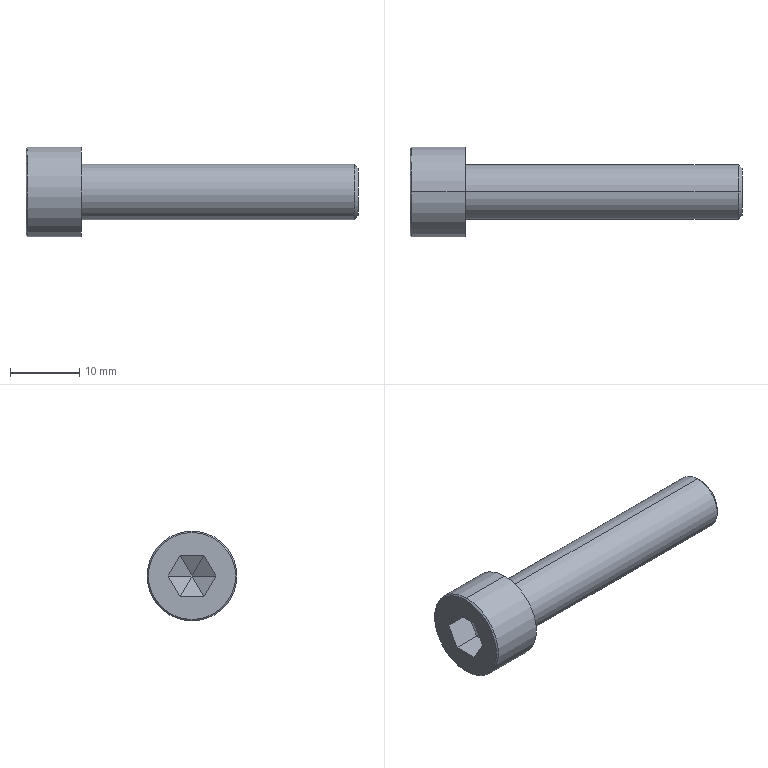Part | NX | features BREP 1 | 1 solid | 23 faces | box 48 x 13 x 13 mm | volume 2924 mm3 | plane 15 | cone 4 | cylinder 4 | commonest cylinder face diameters 8 x2 13 x2
STEP:
#1=CARTESIAN_POINT('',(48.,0.,-3.44));
#2=VERTEX_POINT('',#1);
#3=CARTESIAN_POINT('',(48.,0.,3.44));
#4=VERTEX_POINT('',#3);
#5=CARTESIAN_POINT('',(48.,0.,0.));
#6=DIRECTION('',(1.,0.,0.));
#7=DIRECTION('',(0.,0.,1.));
#8=AXIS2_PLACEMENT_3D('',#5,#6,#7);
#9=CIRCLE('',#8,3.44);
#10=EDGE_CURVE('',#2,#4,#9,.T.);
#11=ORIENTED_EDGE('',*,*,#10,.F.);
#12=CARTESIAN_POINT('',(47.44,0.,-4.));
#13=VERTEX_POINT('',#12);
#14=CARTESIAN_POINT('',(47.44,0.,-4.));
#15=DIRECTION('',(-0.7071,0.,-0.7071));
#16=VECTOR('',#15,1000.);
#17=LINE('',#14,#16);
#18=EDGE_CURVE('',#2,#13,#17,.T.);
#19=ORIENTED_EDGE('',*,*,#18,.T.);
#20=CARTESIAN_POINT('',(47.44,0.,4.));
#21=VERTEX_POINT('',#20);
#22=CARTESIAN_POINT('',(47.44,0.,0.));
#23=DIRECTION('',(-1.,0.,0.));
#24=DIRECTION('',(0.,0.,1.));
#25=AXIS2_PLACEMENT_3D('',#22,#23,#24);
#26=CIRCLE('',#25,4.);
#27=EDGE_CURVE('',#21,#13,#26,.T.);
#28=ORIENTED_EDGE('',*,*,#27,.F.);
#29=CARTESIAN_POINT('',(47.44,0.,4.));
#30=DIRECTION('',(-0.7071,0.,0.7071));
#31=VECTOR('',#30,1000.);
#32=LINE('',#29,#31);
#33=EDGE_CURVE('',#4,#21,#32,.T.);
#34=ORIENTED_EDGE('',*,*,#33,.F.);
#35=EDGE_LOOP('',(#11,#19,#28,#34));
#36=FACE_BOUND('',#35,.T.);
#37=CARTESIAN_POINT('',(47.44,0.,0.));
#38=DIRECTION('',(-1.,0.,0.));
#39=DIRECTION('',(0.,0.,-1.));
#40=AXIS2_PLACEMENT_3D('',#37,#38,#39);
#41=CONICAL_SURFACE('',#40,4.,0.7854);
#42=ADVANCED_FACE('',(#36),#41,.T.);
#43=CARTESIAN_POINT('',(0.,0.,6.3));
#44=VERTEX_POINT('',#43);
#45=CARTESIAN_POINT('',(0.,0.,-6.3));
#46=VERTEX_POINT('',#45);
#47=CARTESIAN_POINT('',(0.,0.,0.));
#48=DIRECTION('',(-1.,0.,0.));
#49=DIRECTION('',(0.,0.,-1.));
#50=AXIS2_PLACEMENT_3D('',#47,#48,#49);
#51=CIRCLE('',#50,6.3);
#52=EDGE_CURVE('',#44,#46,#51,.T.);
#53=ORIENTED_EDGE('',*,*,#52,.F.);
#54=CARTESIAN_POINT('',(0.2,0.,6.5));
#55=VERTEX_POINT('',#54);
#56=CARTESIAN_POINT('',(0.,0.,6.3));
#57=DIRECTION('',(0.7071,0.,0.7071));
#58=VECTOR('',#57,1000.);
#59=LINE('',#56,#58);
#60=EDGE_CURVE('',#55,#44,#59,.F.);
#61=ORIENTED_EDGE('',*,*,#60,.F.);
#62=CARTESIAN_POINT('',(0.2,0.,-6.5));
#63=VERTEX_POINT('',#62);
#64=CARTESIAN_POINT('',(0.2,0.,0.));
#65=DIRECTION('',(1.,0.,0.));
#66=DIRECTION('',(0.,0.,-1.));
#67=AXIS2_PLACEMENT_3D('',#64,#65,#66);
#68=CIRCLE('',#67,6.5);
#69=EDGE_CURVE('',#63,#55,#68,.T.);
#70=ORIENTED_EDGE('',*,*,#69,.F.);
#71=CARTESIAN_POINT('',(0.,0.,-6.3));
#72=DIRECTION('',(0.7071,0.,-0.7071));
#73=VECTOR('',#72,1000.);
#74=LINE('',#71,#73);
#75=EDGE_CURVE('',#63,#46,#74,.F.);
#76=ORIENTED_EDGE('',*,*,#75,.T.);
#77=EDGE_LOOP('',(#53,#61,#70,#76));
#78=FACE_BOUND('',#77,.T.);
#79=CARTESIAN_POINT('',(0.,0.,0.));
#80=DIRECTION('',(1.,0.,0.));
#81=DIRECTION('',(0.,0.,1.));
#82=AXIS2_PLACEMENT_3D('',#79,#80,#81);
#83=CONICAL_SURFACE('',#82,6.3,0.7854);
#84=ADVANCED_FACE('',(#78),#83,.T.);
#85=ORIENTED_EDGE('',*,*,#27,.T.);
#86=CARTESIAN_POINT('',(8.,0.,-4.));
#87=VERTEX_POINT('',#86);
#88=CARTESIAN_POINT('',(0.,0.,-4.));
#89=DIRECTION('',(-1.,0.,0.));
#90=VECTOR('',#89,1000.);
#91=LINE('',#88,#90);
#92=EDGE_CURVE('',#13,#87,#91,.T.);
#93=ORIENTED_EDGE('',*,*,#92,.T.);
#94=CARTESIAN_POINT('',(8.,0.,4.));
#95=VERTEX_POINT('',#94);
#96=CARTESIAN_POINT('',(8.,0.,0.));
#97=DIRECTION('',(-1.,0.,0.));
#98=DIRECTION('',(0.,0.,1.));
#99=AXIS2_PLACEMENT_3D('',#96,#97,#98);
#100=CIRCLE('',#99,4.);
#101=EDGE_CURVE('',#95,#87,#100,.T.);
#102=ORIENTED_EDGE('',*,*,#101,.F.);
#103=CARTESIAN_POINT('',(0.,0.,4.));
#104=DIRECTION('',(-1.,0.,0.));
#105=VECTOR('',#104,1000.);
#106=LINE('',#103,#105);
#107=EDGE_CURVE('',#21,#95,#106,.T.);
#108=ORIENTED_EDGE('',*,*,#107,.F.);
#109=EDGE_LOOP('',(#85,#93,#102,#108));
#110=FACE_BOUND('',#109,.T.);
#111=CARTESIAN_POINT('',(0.,0.,0.));
#112=DIRECTION('',(-1.,0.,0.));
#113=DIRECTION('',(0.,0.,-1.));
#114=AXIS2_PLACEMENT_3D('',#111,#112,#113);
#115=CYLINDRICAL_SURFACE('',#114,4.);
#116=ADVANCED_FACE('',(#110),#115,.T.);
#117=CARTESIAN_POINT('',(8.,0.,6.5));
#118=VERTEX_POINT('',#117);
#119=CARTESIAN_POINT('',(8.,0.,-6.5));
#120=VERTEX_POINT('',#119);
#121=CARTESIAN_POINT('',(8.,0.,0.));
#122=DIRECTION('',(-1.,0.,0.));
#123=DIRECTION('',(0.,0.,1.));
#124=AXIS2_PLACEMENT_3D('',#121,#122,#123);
#125=CIRCLE('',#124,6.5);
#126=EDGE_CURVE('',#118,#120,#125,.T.);
#127=ORIENTED_EDGE('',*,*,#126,.T.);
#128=CARTESIAN_POINT('',(0.,0.,-6.5));
#129=DIRECTION('',(-1.,0.,0.));
#130=VECTOR('',#129,1000.);
#131=LINE('',#128,#130);
#132=EDGE_CURVE('',#120,#63,#131,.T.);
#133=ORIENTED_EDGE('',*,*,#132,.T.);
#134=ORIENTED_EDGE('',*,*,#69,.T.);
#135=CARTESIAN_POINT('',(0.,0.,6.5));
#136=DIRECTION('',(-1.,0.,0.));
#137=VECTOR('',#136,1000.);
#138=LINE('',#135,#137);
#139=EDGE_CURVE('',#118,#55,#138,.T.);
#140=ORIENTED_EDGE('',*,*,#139,.F.);
#141=EDGE_LOOP('',(#127,#133,#134,#140));
#142=FACE_BOUND('',#141,.T.);
#143=CARTESIAN_POINT('',(0.,0.,0.));
#144=DIRECTION('',(-1.,0.,0.));
#145=DIRECTION('',(0.,0.,-1.));
#146=AXIS2_PLACEMENT_3D('',#143,#144,#145);
#147=CYLINDRICAL_SURFACE('',#146,6.5);
#148=ADVANCED_FACE('',(#142),#147,.T.);
#149=CARTESIAN_POINT('',(0.,0.,0.));
#150=DIRECTION('',(-1.,0.,0.));
#151=DIRECTION('',(0.,0.,-1.));
#152=AXIS2_PLACEMENT_3D('',#149,#150,#151);
#153=CIRCLE('',#152,6.3);
#154=EDGE_CURVE('',#46,#44,#153,.T.);
#155=ORIENTED_EDGE('',*,*,#154,.T.);
#156=ORIENTED_EDGE('',*,*,#52,.T.);
#157=EDGE_LOOP('',(#155,#156));
#158=FACE_BOUND('',#157,.T.);
#159=CARTESIAN_POINT('',(0.,1.732,-3.));
#160=VERTEX_POINT('',#159);
#161=CARTESIAN_POINT('',(0.,3.464,0.));
#162=VERTEX_POINT('',#161);
#163=CARTESIAN_POINT('',(0.,1.732,-3.));
#164=DIRECTION('',(0.,0.5,0.866));
#165=VECTOR('',#164,1000.);
#166=LINE('',#163,#165);
#167=EDGE_CURVE('',#160,#162,#166,.T.);
#168=ORIENTED_EDGE('',*,*,#167,.T.);
#169=CARTESIAN_POINT('',(0.,1.732,3.));
#170=VERTEX_POINT('',#169);
#171=CARTESIAN_POINT('',(0.,3.464,0.));
#172=DIRECTION('',(0.,-0.5,0.866));
#173=VECTOR('',#172,1000.);
#174=LINE('',#171,#173);
#175=EDGE_CURVE('',#162,#170,#174,.T.);
#176=ORIENTED_EDGE('',*,*,#175,.T.);
#177=CARTESIAN_POINT('',(0.,-1.732,3.));
#178=VERTEX_POINT('',#177);
#179=CARTESIAN_POINT('',(0.,1.732,3.));
#180=DIRECTION('',(0.,-1.,0.));
#181=VECTOR('',#180,1000.);
#182=LINE('',#179,#181);
#183=EDGE_CURVE('',#170,#178,#182,.T.);
#184=ORIENTED_EDGE('',*,*,#183,.T.);
#185=CARTESIAN_POINT('',(0.,-3.464,0.));
#186=VERTEX_POINT('',#185);
#187=CARTESIAN_POINT('',(0.,-1.732,3.));
#188=DIRECTION('',(0.,-0.5,-0.866));
#189=VECTOR('',#188,1000.);
#190=LINE('',#187,#189);
#191=EDGE_CURVE('',#178,#186,#190,.T.);
#192=ORIENTED_EDGE('',*,*,#191,.T.);
#193=CARTESIAN_POINT('',(0.,-1.732,-3.));
#194=VERTEX_POINT('',#193);
#195=CARTESIAN_POINT('',(0.,-3.464,0.));
#196=DIRECTION('',(0.,0.5,-0.866));
#197=VECTOR('',#196,1000.);
#198=LINE('',#195,#197);
#199=EDGE_CURVE('',#186,#194,#198,.T.);
#200=ORIENTED_EDGE('',*,*,#199,.T.);
#201=CARTESIAN_POINT('',(0.,-1.732,-3.));
#202=DIRECTION('',(0.,1.,0.));
#203=VECTOR('',#202,1000.);
#204=LINE('',#201,#203);
#205=EDGE_CURVE('',#194,#160,#204,.T.);
#206=ORIENTED_EDGE('',*,*,#205,.T.);
#207=EDGE_LOOP('',(#168,#176,#184,#192,#200,#206));
#208=FACE_BOUND('',#207,.T.);
#209=CARTESIAN_POINT('',(0.,0.,0.));
#210=DIRECTION('',(1.,0.,0.));
#211=DIRECTION('',(0.,0.,1.));
#212=AXIS2_PLACEMENT_3D('',#209,#210,#211);
#213=PLANE('',#212);
#214=ADVANCED_FACE('',(#158,#208),#213,.F.);
#215=ORIENTED_EDGE('',*,*,#132,.F.);
#216=CARTESIAN_POINT('',(8.,0.,0.));
#217=DIRECTION('',(-1.,0.,0.));
#218=DIRECTION('',(0.,0.,1.));
#219=AXIS2_PLACEMENT_3D('',#216,#217,#218);
#220=CIRCLE('',#219,6.5);
#221=EDGE_CURVE('',#120,#118,#220,.T.);
#222=ORIENTED_EDGE('',*,*,#221,.T.);
#223=ORIENTED_EDGE('',*,*,#139,.T.);
#224=CARTESIAN_POINT('',(0.2,0.,0.));
#225=DIRECTION('',(1.,0.,0.));
#226=DIRECTION('',(0.,0.,-1.));
#227=AXIS2_PLACEMENT_3D('',#224,#225,#226);
#228=CIRCLE('',#227,6.5);
#229=EDGE_CURVE('',#55,#63,#228,.T.);
#230=ORIENTED_EDGE('',*,*,#229,.T.);
#231=EDGE_LOOP('',(#215,#222,#223,#230));
#232=FACE_BOUND('',#231,.T.);
#233=CARTESIAN_POINT('',(0.,0.,0.));
#234=DIRECTION('',(-1.,0.,0.));
#235=DIRECTION('',(0.,0.,-1.));
#236=AXIS2_PLACEMENT_3D('',#233,#234,#235);
#237=CYLINDRICAL_SURFACE('',#236,6.5);
#238=ADVANCED_FACE('',(#232),#237,.T.);
#239=ORIENTED_EDGE('',*,*,#126,.F.);
#240=ORIENTED_EDGE('',*,*,#221,.F.);
#241=EDGE_LOOP('',(#239,#240));
#242=FACE_BOUND('',#241,.T.);
#243=ORIENTED_EDGE('',*,*,#101,.T.);
#244=CARTESIAN_POINT('',(8.,0.,0.));
#245=DIRECTION('',(-1.,0.,0.));
#246=DIRECTION('',(0.,0.,1.));
#247=AXIS2_PLACEMENT_3D('',#244,#245,#246);
#248=CIRCLE('',#247,4.);
#249=EDGE_CURVE('',#87,#95,#248,.T.);
#250=ORIENTED_EDGE('',*,*,#249,.T.);
#251=EDGE_LOOP('',(#243,#250));
#252=FACE_BOUND('',#251,.T.);
#253=CARTESIAN_POINT('',(8.,6.5,0.));
#254=DIRECTION('',(-1.,0.,0.));
#255=DIRECTION('',(0.,0.,-1.));
#256=AXIS2_PLACEMENT_3D('',#253,#254,#255);
#257=PLANE('',#256);
#258=ADVANCED_FACE('',(#242,#252),#257,.F.);
#259=ORIENTED_EDGE('',*,*,#92,.F.);
#260=CARTESIAN_POINT('',(47.44,0.,0.));
#261=DIRECTION('',(-1.,0.,0.));
#262=DIRECTION('',(0.,0.,1.));
#263=AXIS2_PLACEMENT_3D('',#260,#261,#262);
#264=CIRCLE('',#263,4.);
#265=EDGE_CURVE('',#13,#21,#264,.T.);
#266=ORIENTED_EDGE('',*,*,#265,.T.);
#267=ORIENTED_EDGE('',*,*,#107,.T.);
#268=ORIENTED_EDGE('',*,*,#249,.F.);
#269=EDGE_LOOP('',(#259,#266,#267,#268));
#270=FACE_BOUND('',#269,.T.);
#271=CARTESIAN_POINT('',(0.,0.,0.));
#272=DIRECTION('',(-1.,0.,0.));
#273=DIRECTION('',(0.,0.,-1.));
#274=AXIS2_PLACEMENT_3D('',#271,#272,#273);
#275=CYLINDRICAL_SURFACE('',#274,4.);
#276=ADVANCED_FACE('',(#270),#275,.T.);
#277=CARTESIAN_POINT('',(48.,0.,0.));
#278=DIRECTION('',(1.,0.,0.));
#279=DIRECTION('',(0.,0.,1.));
#280=AXIS2_PLACEMENT_3D('',#277,#278,#279);
#281=CIRCLE('',#280,3.44);
#282=EDGE_CURVE('',#4,#2,#281,.T.);
#283=ORIENTED_EDGE('',*,*,#282,.T.);
#284=ORIENTED_EDGE('',*,*,#10,.T.);
#285=EDGE_LOOP('',(#283,#284));
#286=FACE_BOUND('',#285,.T.);
#287=CARTESIAN_POINT('',(48.,4.,0.));
#288=DIRECTION('',(-1.,0.,0.));
#289=DIRECTION('',(0.,0.,-1.));
#290=AXIS2_PLACEMENT_3D('',#287,#288,#289);
#291=PLANE('',#290);
#292=ADVANCED_FACE('',(#286),#291,.F.);
#293=ORIENTED_EDGE('',*,*,#167,.F.);
#294=CARTESIAN_POINT('',(4.,1.732,-3.));
#295=VERTEX_POINT('',#294);
#296=CARTESIAN_POINT('',(4.,1.732,-3.));
#297=DIRECTION('',(-1.,0.,0.));
#298=VECTOR('',#297,1000.);
#299=LINE('',#296,#298);
#300=EDGE_CURVE('',#295,#160,#299,.T.);
#301=ORIENTED_EDGE('',*,*,#300,.F.);
#302=CARTESIAN_POINT('',(4.,3.464,0.));
#303=VERTEX_POINT('',#302);
#304=CARTESIAN_POINT('',(4.,1.732,-3.));
#305=DIRECTION('',(0.,0.5,0.866));
#306=VECTOR('',#305,1000.);
#307=LINE('',#304,#306);
#308=EDGE_CURVE('',#295,#303,#307,.T.);
#309=ORIENTED_EDGE('',*,*,#308,.T.);
#310=CARTESIAN_POINT('',(4.,3.464,0.));
#311=DIRECTION('',(-1.,0.,0.));
#312=VECTOR('',#311,1000.);
#313=LINE('',#310,#312);
#314=EDGE_CURVE('',#303,#162,#313,.T.);
#315=ORIENTED_EDGE('',*,*,#314,.T.);
#316=EDGE_LOOP('',(#293,#301,#309,#315));
#317=FACE_BOUND('',#316,.T.);
#318=CARTESIAN_POINT('',(4.,1.732,-3.));
#319=DIRECTION('',(0.,-0.866,0.5));
#320=DIRECTION('',(0.,0.5,0.866));
#321=AXIS2_PLACEMENT_3D('',#318,#319,#320);
#322=PLANE('',#321);
#323=ADVANCED_FACE('',(#317),#322,.T.);
#324=ORIENTED_EDGE('',*,*,#175,.F.);
#325=ORIENTED_EDGE('',*,*,#314,.F.);
#326=CARTESIAN_POINT('',(4.,1.732,3.));
#327=VERTEX_POINT('',#326);
#328=CARTESIAN_POINT('',(4.,3.464,0.));
#329=DIRECTION('',(0.,-0.5,0.866));
#330=VECTOR('',#329,1000.);
#331=LINE('',#328,#330);
#332=EDGE_CURVE('',#303,#327,#331,.T.);
#333=ORIENTED_EDGE('',*,*,#332,.T.);
#334=CARTESIAN_POINT('',(4.,1.732,3.));
#335=DIRECTION('',(-1.,0.,0.));
#336=VECTOR('',#335,1000.);
#337=LINE('',#334,#336);
#338=EDGE_CURVE('',#327,#170,#337,.T.);
#339=ORIENTED_EDGE('',*,*,#338,.T.);
#340=EDGE_LOOP('',(#324,#325,#333,#339));
#341=FACE_BOUND('',#340,.T.);
#342=CARTESIAN_POINT('',(4.,3.464,0.));
#343=DIRECTION('',(0.,-0.866,-0.5));
#344=DIRECTION('',(0.,-0.5,0.866));
#345=AXIS2_PLACEMENT_3D('',#342,#343,#344);
#346=PLANE('',#345);
#347=ADVANCED_FACE('',(#341),#346,.T.);
#348=ORIENTED_EDGE('',*,*,#183,.F.);
#349=ORIENTED_EDGE('',*,*,#338,.F.);
#350=CARTESIAN_POINT('',(4.,-1.732,3.));
#351=VERTEX_POINT('',#350);
#352=CARTESIAN_POINT('',(4.,1.732,3.));
#353=DIRECTION('',(0.,-1.,0.));
#354=VECTOR('',#353,1000.);
#355=LINE('',#352,#354);
#356=EDGE_CURVE('',#327,#351,#355,.T.);
#357=ORIENTED_EDGE('',*,*,#356,.T.);
#358=CARTESIAN_POINT('',(4.,-1.732,3.));
#359=DIRECTION('',(-1.,0.,0.));
#360=VECTOR('',#359,1000.);
#361=LINE('',#358,#360);
#362=EDGE_CURVE('',#351,#178,#361,.T.);
#363=ORIENTED_EDGE('',*,*,#362,.T.);
#364=EDGE_LOOP('',(#348,#349,#357,#363));
#365=FACE_BOUND('',#364,.T.);
#366=CARTESIAN_POINT('',(4.,1.732,3.));
#367=DIRECTION('',(0.,0.,-1.));
#368=DIRECTION('',(1.,0.,0.));
#369=AXIS2_PLACEMENT_3D('',#366,#367,#368);
#370=PLANE('',#369);
#371=ADVANCED_FACE('',(#365),#370,.T.);
#372=ORIENTED_EDGE('',*,*,#191,.F.);
#373=ORIENTED_EDGE('',*,*,#362,.F.);
#374=CARTESIAN_POINT('',(4.,-3.464,0.));
#375=VERTEX_POINT('',#374);
#376=CARTESIAN_POINT('',(4.,-1.732,3.));
#377=DIRECTION('',(0.,-0.5,-0.866));
#378=VECTOR('',#377,1000.);
#379=LINE('',#376,#378);
#380=EDGE_CURVE('',#351,#375,#379,.T.);
#381=ORIENTED_EDGE('',*,*,#380,.T.);
#382=CARTESIAN_POINT('',(4.,-3.464,0.));
#383=DIRECTION('',(-1.,0.,0.));
#384=VECTOR('',#383,1000.);
#385=LINE('',#382,#384);
#386=EDGE_CURVE('',#375,#186,#385,.T.);
#387=ORIENTED_EDGE('',*,*,#386,.T.);
#388=EDGE_LOOP('',(#372,#373,#381,#387));
#389=FACE_BOUND('',#388,.T.);
#390=CARTESIAN_POINT('',(4.,-1.732,3.));
#391=DIRECTION('',(0.,0.866,-0.5));
#392=DIRECTION('',(0.,-0.5,-0.866));
#393=AXIS2_PLACEMENT_3D('',#390,#391,#392);
#394=PLANE('',#393);
#395=ADVANCED_FACE('',(#389),#394,.T.);
#396=ORIENTED_EDGE('',*,*,#199,.F.);
#397=ORIENTED_EDGE('',*,*,#386,.F.);
#398=CARTESIAN_POINT('',(4.,-1.732,-3.));
#399=VERTEX_POINT('',#398);
#400=CARTESIAN_POINT('',(4.,-3.464,0.));
#401=DIRECTION('',(0.,0.5,-0.866));
#402=VECTOR('',#401,1000.);
#403=LINE('',#400,#402);
#404=EDGE_CURVE('',#375,#399,#403,.T.);
#405=ORIENTED_EDGE('',*,*,#404,.T.);
#406=CARTESIAN_POINT('',(4.,-1.732,-3.));
#407=DIRECTION('',(-1.,0.,0.));
#408=VECTOR('',#407,1000.);
#409=LINE('',#406,#408);
#410=EDGE_CURVE('',#399,#194,#409,.T.);
#411=ORIENTED_EDGE('',*,*,#410,.T.);
#412=EDGE_LOOP('',(#396,#397,#405,#411));
#413=FACE_BOUND('',#412,.T.);
#414=CARTESIAN_POINT('',(4.,-3.464,0.));
#415=DIRECTION('',(0.,0.866,0.5));
#416=DIRECTION('',(0.,0.5,-0.866));
#417=AXIS2_PLACEMENT_3D('',#414,#415,#416);
#418=PLANE('',#417);
#419=ADVANCED_FACE('',(#413),#418,.T.);
#420=ORIENTED_EDGE('',*,*,#205,.F.);
#421=ORIENTED_EDGE('',*,*,#410,.F.);
#422=CARTESIAN_POINT('',(4.,-1.732,-3.));
#423=DIRECTION('',(0.,1.,0.));
#424=VECTOR('',#423,1000.);
#425=LINE('',#422,#424);
#426=EDGE_CURVE('',#399,#295,#425,.T.);
#427=ORIENTED_EDGE('',*,*,#426,.T.);
#428=ORIENTED_EDGE('',*,*,#300,.T.);
#429=EDGE_LOOP('',(#420,#421,#427,#428));
#430=FACE_BOUND('',#429,.T.);
#431=CARTESIAN_POINT('',(4.,-1.732,-3.));
#432=DIRECTION('',(0.,0.,1.));
#433=DIRECTION('',(-1.,0.,0.));
#434=AXIS2_PLACEMENT_3D('',#431,#432,#433);
#435=PLANE('',#434);
#436=ADVANCED_FACE('',(#430),#435,.T.);
#437=ORIENTED_EDGE('',*,*,#60,.T.);
#438=ORIENTED_EDGE('',*,*,#154,.F.);
#439=ORIENTED_EDGE('',*,*,#75,.F.);
#440=ORIENTED_EDGE('',*,*,#229,.F.);
#441=EDGE_LOOP('',(#437,#438,#439,#440));
#442=FACE_BOUND('',#441,.T.);
#443=CARTESIAN_POINT('',(0.,0.,0.));
#444=DIRECTION('',(1.,0.,0.));
#445=DIRECTION('',(0.,0.,1.));
#446=AXIS2_PLACEMENT_3D('',#443,#444,#445);
#447=CONICAL_SURFACE('',#446,6.3,0.7854);
#448=ADVANCED_FACE('',(#442),#447,.T.);
#449=ORIENTED_EDGE('',*,*,#18,.F.);
#450=ORIENTED_EDGE('',*,*,#282,.F.);
#451=ORIENTED_EDGE('',*,*,#33,.T.);
#452=ORIENTED_EDGE('',*,*,#265,.F.);
#453=EDGE_LOOP('',(#449,#450,#451,#452));
#454=FACE_BOUND('',#453,.T.);
#455=CARTESIAN_POINT('',(47.44,0.,0.));
#456=DIRECTION('',(-1.,0.,0.));
#457=DIRECTION('',(0.,0.,-1.));
#458=AXIS2_PLACEMENT_3D('',#455,#456,#457);
#459=CONICAL_SURFACE('',#458,4.,0.7854);
#460=ADVANCED_FACE('',(#454),#459,.T.);
#461=ORIENTED_EDGE('',*,*,#380,.F.);
#462=CARTESIAN_POINT('',(5.803,0.,0.));
#463=VERTEX_POINT('',#462);
#464=CARTESIAN_POINT('',(4.709,-1.051,1.82));
#465=DIRECTION('',(-0.4616,-0.4435,0.7682));
#466=VECTOR('',#465,1000.);
#467=LINE('',#464,#466);
#468=EDGE_CURVE('',#463,#351,#467,.T.);
#469=ORIENTED_EDGE('',*,*,#468,.F.);
#470=CARTESIAN_POINT('',(4.709,-2.101,0.));
#471=DIRECTION('',(-0.4616,-0.8871,0.));
#472=VECTOR('',#471,1000.);
#473=LINE('',#470,#472);
#474=EDGE_CURVE('',#463,#375,#473,.T.);
#475=ORIENTED_EDGE('',*,*,#474,.T.);
#476=EDGE_LOOP('',(#461,#469,#475));
#477=FACE_BOUND('',#476,.T.);
#478=CARTESIAN_POINT('',(4.,-3.464,0.));
#479=DIRECTION('',(0.8572,-0.446,0.2575));
#480=DIRECTION('',(-0.4616,-0.8871,0.));
#481=AXIS2_PLACEMENT_3D('',#478,#479,#480);
#482=PLANE('',#481);
#483=ADVANCED_FACE('',(#477),#482,.F.);
#484=ORIENTED_EDGE('',*,*,#404,.F.);
#485=ORIENTED_EDGE('',*,*,#474,.F.);
#486=CARTESIAN_POINT('',(4.709,-1.051,-1.82));
#487=DIRECTION('',(-0.4616,-0.4435,-0.7682));
#488=VECTOR('',#487,1000.);
#489=LINE('',#486,#488);
#490=EDGE_CURVE('',#463,#399,#489,.T.);
#491=ORIENTED_EDGE('',*,*,#490,.T.);
#492=EDGE_LOOP('',(#484,#485,#491));
#493=FACE_BOUND('',#492,.T.);
#494=CARTESIAN_POINT('',(4.,-1.732,-3.));
#495=DIRECTION('',(0.8572,-0.446,-0.2575));
#496=DIRECTION('',(-0.4616,-0.8871,0.));
#497=AXIS2_PLACEMENT_3D('',#494,#495,#496);
#498=PLANE('',#497);
#499=ADVANCED_FACE('',(#493),#498,.F.);
#500=ORIENTED_EDGE('',*,*,#426,.F.);
#501=ORIENTED_EDGE('',*,*,#490,.F.);
#502=CARTESIAN_POINT('',(4.709,1.051,-1.82));
#503=DIRECTION('',(-0.4616,0.4435,-0.7682));
#504=VECTOR('',#503,1000.);
#505=LINE('',#502,#504);
#506=EDGE_CURVE('',#463,#295,#505,.T.);
#507=ORIENTED_EDGE('',*,*,#506,.T.);
#508=EDGE_LOOP('',(#500,#501,#507));
#509=FACE_BOUND('',#508,.T.);
#510=CARTESIAN_POINT('',(4.,1.732,-3.));
#511=DIRECTION('',(0.8572,0.,-0.515));
#512=DIRECTION('',(0.515,0.,0.8572));
#513=AXIS2_PLACEMENT_3D('',#510,#511,#512);
#514=PLANE('',#513);
#515=ADVANCED_FACE('',(#509),#514,.F.);
#516=ORIENTED_EDGE('',*,*,#308,.F.);
#517=ORIENTED_EDGE('',*,*,#506,.F.);
#518=CARTESIAN_POINT('',(4.709,2.101,0.));
#519=DIRECTION('',(-0.4616,0.8871,0.));
#520=VECTOR('',#519,1000.);
#521=LINE('',#518,#520);
#522=EDGE_CURVE('',#463,#303,#521,.T.);
#523=ORIENTED_EDGE('',*,*,#522,.T.);
#524=EDGE_LOOP('',(#516,#517,#523));
#525=FACE_BOUND('',#524,.T.);
#526=CARTESIAN_POINT('',(4.,3.464,0.));
#527=DIRECTION('',(0.8572,0.446,-0.2575));
#528=DIRECTION('',(0.4616,-0.8871,0.));
#529=AXIS2_PLACEMENT_3D('',#526,#527,#528);
#530=PLANE('',#529);
#531=ADVANCED_FACE('',(#525),#530,.F.);
#532=ORIENTED_EDGE('',*,*,#332,.F.);
#533=ORIENTED_EDGE('',*,*,#522,.F.);
#534=CARTESIAN_POINT('',(4.709,1.051,1.82));
#535=DIRECTION('',(-0.4616,0.4435,0.7682));
#536=VECTOR('',#535,1000.);
#537=LINE('',#534,#536);
#538=EDGE_CURVE('',#463,#327,#537,.T.);
#539=ORIENTED_EDGE('',*,*,#538,.T.);
#540=EDGE_LOOP('',(#532,#533,#539));
#541=FACE_BOUND('',#540,.T.);
#542=CARTESIAN_POINT('',(4.,1.732,3.));
#543=DIRECTION('',(0.8572,0.446,0.2575));
#544=DIRECTION('',(0.4616,-0.8871,0.));
#545=AXIS2_PLACEMENT_3D('',#542,#543,#544);
#546=PLANE('',#545);
#547=ADVANCED_FACE('',(#541),#546,.F.);
#548=ORIENTED_EDGE('',*,*,#356,.F.);
#549=ORIENTED_EDGE('',*,*,#538,.F.);
#550=ORIENTED_EDGE('',*,*,#468,.T.);
#551=EDGE_LOOP('',(#548,#549,#550));
#552=FACE_BOUND('',#551,.T.);
#553=CARTESIAN_POINT('',(4.,-1.732,3.));
#554=DIRECTION('',(0.8572,0.,0.515));
#555=DIRECTION('',(-0.515,0.,0.8572));
#556=AXIS2_PLACEMENT_3D('',#553,#554,#555);
#557=PLANE('',#556);
#558=ADVANCED_FACE('',(#552),#557,.F.);
#559=CLOSED_SHELL('',(#42,#84,#116,#148,#214,#238,#258,#276,#292,#323,#347,#371,#395,#419,#436,#448,#460,#483,#499,#515,#531,#547,#558));
#560=MANIFOLD_SOLID_BREP('',#559);
#561=(LENGTH_UNIT()NAMED_UNIT(*)SI_UNIT(.MILLI.,.METRE.));
#562=UNCERTAINTY_MEASURE_WITH_UNIT(LENGTH_MEASURE(0.00001),#561,'','');
#563=(NAMED_UNIT(*)PLANE_ANGLE_UNIT()SI_UNIT($,.RADIAN.));
#564=(NAMED_UNIT(*)SI_UNIT($,.STERADIAN.)SOLID_ANGLE_UNIT());
#565=(GEOMETRIC_REPRESENTATION_CONTEXT(3)GLOBAL_UNCERTAINTY_ASSIGNED_CONTEXT((#562))GLOBAL_UNIT_ASSIGNED_CONTEXT((#561,#563,#564))REPRESENTATION_CONTEXT('',''));
#566=ADVANCED_BREP_SHAPE_REPRESENTATION('',(#560),#565);